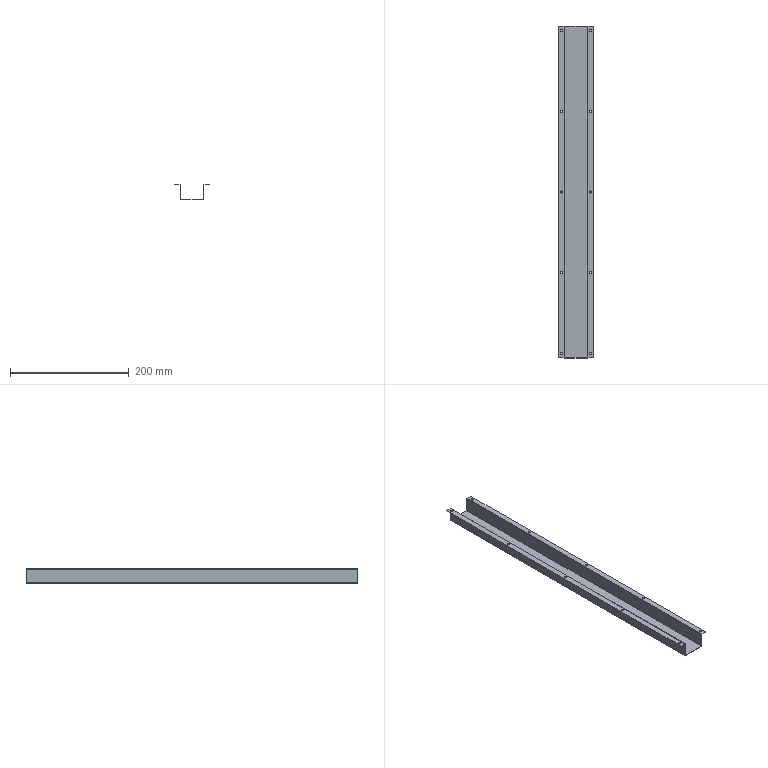Part | SolidWorks | features BaseBody 1 | 1 solid | 42 faces | box 58.8 x 560 x 25 mm | volume 35807 mm3 | cylinder 28 | plane 14 | commonest cylinder face diameters 3.5 x20 0.4 x4 1.6 x4
STEP:
#1=CARTESIAN_POINT('',(322.65,272.,-1.2));
#2=VERTEX_POINT('',#1);
#3=CARTESIAN_POINT('',(326.15,272.,-1.2));
#4=VERTEX_POINT('',#3);
#5=CARTESIAN_POINT('',(324.4,272.,-1.2));
#6=DIRECTION('',(0.,0.,1.));
#7=DIRECTION('',(1.,0.,0.));
#8=AXIS2_PLACEMENT_3D('',#5,#6,#7);
#9=CIRCLE('',#8,1.75);
#10=EDGE_CURVE('',#2,#4,#9,.T.);
#11=ORIENTED_EDGE('',*,*,#10,.F.);
#12=CARTESIAN_POINT('',(322.65,272.,-0.6));
#13=VERTEX_POINT('',#12);
#14=CARTESIAN_POINT('',(322.65,272.,-1.2));
#15=DIRECTION('',(0.,0.,1.));
#16=VECTOR('',#15,1000.);
#17=LINE('',#14,#16);
#18=EDGE_CURVE('',#2,#13,#17,.T.);
#19=ORIENTED_EDGE('',*,*,#18,.T.);
#20=CARTESIAN_POINT('',(326.15,272.,-0.6));
#21=VERTEX_POINT('',#20);
#22=CARTESIAN_POINT('',(324.4,272.,-0.6));
#23=DIRECTION('',(0.,0.,-1.));
#24=DIRECTION('',(1.,0.,0.));
#25=AXIS2_PLACEMENT_3D('',#22,#23,#24);
#26=CIRCLE('',#25,1.75);
#27=EDGE_CURVE('',#21,#13,#26,.T.);
#28=ORIENTED_EDGE('',*,*,#27,.F.);
#29=CARTESIAN_POINT('',(326.15,272.,-1.2));
#30=DIRECTION('',(0.,0.,1.));
#31=VECTOR('',#30,1000.);
#32=LINE('',#29,#31);
#33=EDGE_CURVE('',#4,#21,#32,.T.);
#34=ORIENTED_EDGE('',*,*,#33,.F.);
#35=EDGE_LOOP('',(#11,#19,#28,#34));
#36=FACE_OUTER_BOUND('',#35,.T.);
#37=CARTESIAN_POINT('',(324.4,272.,-1.2));
#38=DIRECTION('',(0.,0.,1.));
#39=DIRECTION('',(1.,0.,0.));
#40=AXIS2_PLACEMENT_3D('',#37,#38,#39);
#41=CYLINDRICAL_SURFACE('',#40,1.75);
#42=ADVANCED_FACE('',(#36),#41,.F.);
#43=CARTESIAN_POINT('',(322.65,0.,-1.2));
#44=VERTEX_POINT('',#43);
#45=CARTESIAN_POINT('',(326.15,0.,-1.2));
#46=VERTEX_POINT('',#45);
#47=CARTESIAN_POINT('',(324.4,0.,-1.2));
#48=DIRECTION('',(0.,0.,1.));
#49=DIRECTION('',(1.,0.,0.));
#50=AXIS2_PLACEMENT_3D('',#47,#48,#49);
#51=CIRCLE('',#50,1.75);
#52=EDGE_CURVE('',#44,#46,#51,.T.);
#53=ORIENTED_EDGE('',*,*,#52,.F.);
#54=CARTESIAN_POINT('',(322.65,0.,-0.6));
#55=VERTEX_POINT('',#54);
#56=CARTESIAN_POINT('',(322.65,0.,-1.2));
#57=DIRECTION('',(0.,0.,1.));
#58=VECTOR('',#57,1000.);
#59=LINE('',#56,#58);
#60=EDGE_CURVE('',#44,#55,#59,.T.);
#61=ORIENTED_EDGE('',*,*,#60,.T.);
#62=CARTESIAN_POINT('',(326.15,0.,-0.6));
#63=VERTEX_POINT('',#62);
#64=CARTESIAN_POINT('',(324.4,0.,-0.6));
#65=DIRECTION('',(0.,0.,-1.));
#66=DIRECTION('',(1.,0.,0.));
#67=AXIS2_PLACEMENT_3D('',#64,#65,#66);
#68=CIRCLE('',#67,1.75);
#69=EDGE_CURVE('',#63,#55,#68,.T.);
#70=ORIENTED_EDGE('',*,*,#69,.F.);
#71=CARTESIAN_POINT('',(326.15,0.,-1.2));
#72=DIRECTION('',(0.,0.,1.));
#73=VECTOR('',#72,1000.);
#74=LINE('',#71,#73);
#75=EDGE_CURVE('',#46,#63,#74,.T.);
#76=ORIENTED_EDGE('',*,*,#75,.F.);
#77=EDGE_LOOP('',(#53,#61,#70,#76));
#78=FACE_OUTER_BOUND('',#77,.T.);
#79=CARTESIAN_POINT('',(324.4,0.,-1.2));
#80=DIRECTION('',(0.,0.,1.));
#81=DIRECTION('',(1.,0.,0.));
#82=AXIS2_PLACEMENT_3D('',#79,#80,#81);
#83=CYLINDRICAL_SURFACE('',#82,1.75);
#84=ADVANCED_FACE('',(#78),#83,.F.);
#85=CARTESIAN_POINT('',(322.65,136.,-1.2));
#86=VERTEX_POINT('',#85);
#87=CARTESIAN_POINT('',(326.15,136.,-1.2));
#88=VERTEX_POINT('',#87);
#89=CARTESIAN_POINT('',(324.4,136.,-1.2));
#90=DIRECTION('',(0.,0.,1.));
#91=DIRECTION('',(1.,0.,0.));
#92=AXIS2_PLACEMENT_3D('',#89,#90,#91);
#93=CIRCLE('',#92,1.75);
#94=EDGE_CURVE('',#86,#88,#93,.T.);
#95=ORIENTED_EDGE('',*,*,#94,.F.);
#96=CARTESIAN_POINT('',(322.65,136.,-0.6));
#97=VERTEX_POINT('',#96);
#98=CARTESIAN_POINT('',(322.65,136.,-1.2));
#99=DIRECTION('',(0.,0.,1.));
#100=VECTOR('',#99,1000.);
#101=LINE('',#98,#100);
#102=EDGE_CURVE('',#86,#97,#101,.T.);
#103=ORIENTED_EDGE('',*,*,#102,.T.);
#104=CARTESIAN_POINT('',(326.15,136.,-0.6));
#105=VERTEX_POINT('',#104);
#106=CARTESIAN_POINT('',(324.4,136.,-0.6));
#107=DIRECTION('',(0.,0.,-1.));
#108=DIRECTION('',(1.,0.,0.));
#109=AXIS2_PLACEMENT_3D('',#106,#107,#108);
#110=CIRCLE('',#109,1.75);
#111=EDGE_CURVE('',#105,#97,#110,.T.);
#112=ORIENTED_EDGE('',*,*,#111,.F.);
#113=CARTESIAN_POINT('',(326.15,136.,-1.2));
#114=DIRECTION('',(0.,0.,1.));
#115=VECTOR('',#114,1000.);
#116=LINE('',#113,#115);
#117=EDGE_CURVE('',#88,#105,#116,.T.);
#118=ORIENTED_EDGE('',*,*,#117,.F.);
#119=EDGE_LOOP('',(#95,#103,#112,#118));
#120=FACE_OUTER_BOUND('',#119,.T.);
#121=CARTESIAN_POINT('',(324.4,136.,-1.2));
#122=DIRECTION('',(0.,0.,1.));
#123=DIRECTION('',(1.,0.,0.));
#124=AXIS2_PLACEMENT_3D('',#121,#122,#123);
#125=CYLINDRICAL_SURFACE('',#124,1.75);
#126=ADVANCED_FACE('',(#120),#125,.F.);
#127=CARTESIAN_POINT('',(322.65,-272.,-1.2));
#128=VERTEX_POINT('',#127);
#129=CARTESIAN_POINT('',(326.15,-272.,-1.2));
#130=VERTEX_POINT('',#129);
#131=CARTESIAN_POINT('',(324.4,-272.,-1.2));
#132=DIRECTION('',(0.,0.,1.));
#133=DIRECTION('',(1.,0.,0.));
#134=AXIS2_PLACEMENT_3D('',#131,#132,#133);
#135=CIRCLE('',#134,1.75);
#136=EDGE_CURVE('',#128,#130,#135,.T.);
#137=ORIENTED_EDGE('',*,*,#136,.F.);
#138=CARTESIAN_POINT('',(322.65,-272.,-0.6));
#139=VERTEX_POINT('',#138);
#140=CARTESIAN_POINT('',(322.65,-272.,-1.2));
#141=DIRECTION('',(0.,0.,1.));
#142=VECTOR('',#141,1000.);
#143=LINE('',#140,#142);
#144=EDGE_CURVE('',#128,#139,#143,.T.);
#145=ORIENTED_EDGE('',*,*,#144,.T.);
#146=CARTESIAN_POINT('',(326.15,-272.,-0.6));
#147=VERTEX_POINT('',#146);
#148=CARTESIAN_POINT('',(324.4,-272.,-0.6));
#149=DIRECTION('',(0.,0.,-1.));
#150=DIRECTION('',(1.,0.,0.));
#151=AXIS2_PLACEMENT_3D('',#148,#149,#150);
#152=CIRCLE('',#151,1.75);
#153=EDGE_CURVE('',#147,#139,#152,.T.);
#154=ORIENTED_EDGE('',*,*,#153,.F.);
#155=CARTESIAN_POINT('',(326.15,-272.,-1.2));
#156=DIRECTION('',(0.,0.,1.));
#157=VECTOR('',#156,1000.);
#158=LINE('',#155,#157);
#159=EDGE_CURVE('',#130,#147,#158,.T.);
#160=ORIENTED_EDGE('',*,*,#159,.F.);
#161=EDGE_LOOP('',(#137,#145,#154,#160));
#162=FACE_OUTER_BOUND('',#161,.T.);
#163=CARTESIAN_POINT('',(324.4,-272.,-1.2));
#164=DIRECTION('',(0.,0.,1.));
#165=DIRECTION('',(1.,0.,0.));
#166=AXIS2_PLACEMENT_3D('',#163,#164,#165);
#167=CYLINDRICAL_SURFACE('',#166,1.75);
#168=ADVANCED_FACE('',(#162),#167,.F.);
#169=CARTESIAN_POINT('',(322.65,-136.,-1.2));
#170=VERTEX_POINT('',#169);
#171=CARTESIAN_POINT('',(326.15,-136.,-1.2));
#172=VERTEX_POINT('',#171);
#173=CARTESIAN_POINT('',(324.4,-136.,-1.2));
#174=DIRECTION('',(0.,0.,1.));
#175=DIRECTION('',(1.,0.,0.));
#176=AXIS2_PLACEMENT_3D('',#173,#174,#175);
#177=CIRCLE('',#176,1.75);
#178=EDGE_CURVE('',#170,#172,#177,.T.);
#179=ORIENTED_EDGE('',*,*,#178,.F.);
#180=CARTESIAN_POINT('',(322.65,-136.,-0.6));
#181=VERTEX_POINT('',#180);
#182=CARTESIAN_POINT('',(322.65,-136.,-1.2));
#183=DIRECTION('',(0.,0.,1.));
#184=VECTOR('',#183,1000.);
#185=LINE('',#182,#184);
#186=EDGE_CURVE('',#170,#181,#185,.T.);
#187=ORIENTED_EDGE('',*,*,#186,.T.);
#188=CARTESIAN_POINT('',(326.15,-136.,-0.6));
#189=VERTEX_POINT('',#188);
#190=CARTESIAN_POINT('',(324.4,-136.,-0.6));
#191=DIRECTION('',(0.,0.,-1.));
#192=DIRECTION('',(1.,0.,0.));
#193=AXIS2_PLACEMENT_3D('',#190,#191,#192);
#194=CIRCLE('',#193,1.75);
#195=EDGE_CURVE('',#189,#181,#194,.T.);
#196=ORIENTED_EDGE('',*,*,#195,.F.);
#197=CARTESIAN_POINT('',(326.15,-136.,-1.2));
#198=DIRECTION('',(0.,0.,1.));
#199=VECTOR('',#198,1000.);
#200=LINE('',#197,#199);
#201=EDGE_CURVE('',#172,#189,#200,.T.);
#202=ORIENTED_EDGE('',*,*,#201,.F.);
#203=EDGE_LOOP('',(#179,#187,#196,#202));
#204=FACE_OUTER_BOUND('',#203,.T.);
#205=CARTESIAN_POINT('',(324.4,-136.,-1.2));
#206=DIRECTION('',(0.,0.,1.));
#207=DIRECTION('',(1.,0.,0.));
#208=AXIS2_PLACEMENT_3D('',#205,#206,#207);
#209=CYLINDRICAL_SURFACE('',#208,1.75);
#210=ADVANCED_FACE('',(#204),#209,.F.);
#211=CARTESIAN_POINT('',(273.85,-272.,-1.2));
#212=VERTEX_POINT('',#211);
#213=CARTESIAN_POINT('',(277.35,-272.,-1.2));
#214=VERTEX_POINT('',#213);
#215=CARTESIAN_POINT('',(275.6,-272.,-1.2));
#216=DIRECTION('',(0.,0.,1.));
#217=DIRECTION('',(1.,0.,0.));
#218=AXIS2_PLACEMENT_3D('',#215,#216,#217);
#219=CIRCLE('',#218,1.75);
#220=EDGE_CURVE('',#212,#214,#219,.T.);
#221=ORIENTED_EDGE('',*,*,#220,.F.);
#222=CARTESIAN_POINT('',(273.85,-272.,-0.6));
#223=VERTEX_POINT('',#222);
#224=CARTESIAN_POINT('',(273.85,-272.,-1.2));
#225=DIRECTION('',(0.,0.,1.));
#226=VECTOR('',#225,1000.);
#227=LINE('',#224,#226);
#228=EDGE_CURVE('',#212,#223,#227,.T.);
#229=ORIENTED_EDGE('',*,*,#228,.T.);
#230=CARTESIAN_POINT('',(277.35,-272.,-0.6));
#231=VERTEX_POINT('',#230);
#232=CARTESIAN_POINT('',(275.6,-272.,-0.6));
#233=DIRECTION('',(0.,0.,-1.));
#234=DIRECTION('',(1.,0.,0.));
#235=AXIS2_PLACEMENT_3D('',#232,#233,#234);
#236=CIRCLE('',#235,1.75);
#237=EDGE_CURVE('',#231,#223,#236,.T.);
#238=ORIENTED_EDGE('',*,*,#237,.F.);
#239=CARTESIAN_POINT('',(277.35,-272.,-1.2));
#240=DIRECTION('',(0.,0.,1.));
#241=VECTOR('',#240,1000.);
#242=LINE('',#239,#241);
#243=EDGE_CURVE('',#214,#231,#242,.T.);
#244=ORIENTED_EDGE('',*,*,#243,.F.);
#245=EDGE_LOOP('',(#221,#229,#238,#244));
#246=FACE_OUTER_BOUND('',#245,.T.);
#247=CARTESIAN_POINT('',(275.6,-272.,-1.2));
#248=DIRECTION('',(0.,0.,1.));
#249=DIRECTION('',(1.,0.,0.));
#250=AXIS2_PLACEMENT_3D('',#247,#248,#249);
#251=CYLINDRICAL_SURFACE('',#250,1.75);
#252=ADVANCED_FACE('',(#246),#251,.F.);
#253=CARTESIAN_POINT('',(273.85,136.,-1.2));
#254=VERTEX_POINT('',#253);
#255=CARTESIAN_POINT('',(277.35,136.,-1.2));
#256=VERTEX_POINT('',#255);
#257=CARTESIAN_POINT('',(275.6,136.,-1.2));
#258=DIRECTION('',(0.,0.,1.));
#259=DIRECTION('',(1.,0.,0.));
#260=AXIS2_PLACEMENT_3D('',#257,#258,#259);
#261=CIRCLE('',#260,1.75);
#262=EDGE_CURVE('',#254,#256,#261,.T.);
#263=ORIENTED_EDGE('',*,*,#262,.F.);
#264=CARTESIAN_POINT('',(273.85,136.,-0.6));
#265=VERTEX_POINT('',#264);
#266=CARTESIAN_POINT('',(273.85,136.,-1.2));
#267=DIRECTION('',(0.,0.,1.));
#268=VECTOR('',#267,1000.);
#269=LINE('',#266,#268);
#270=EDGE_CURVE('',#254,#265,#269,.T.);
#271=ORIENTED_EDGE('',*,*,#270,.T.);
#272=CARTESIAN_POINT('',(277.35,136.,-0.6));
#273=VERTEX_POINT('',#272);
#274=CARTESIAN_POINT('',(275.6,136.,-0.6));
#275=DIRECTION('',(0.,0.,-1.));
#276=DIRECTION('',(1.,0.,0.));
#277=AXIS2_PLACEMENT_3D('',#274,#275,#276);
#278=CIRCLE('',#277,1.75);
#279=EDGE_CURVE('',#273,#265,#278,.T.);
#280=ORIENTED_EDGE('',*,*,#279,.F.);
#281=CARTESIAN_POINT('',(277.35,136.,-1.2));
#282=DIRECTION('',(0.,0.,1.));
#283=VECTOR('',#282,1000.);
#284=LINE('',#281,#283);
#285=EDGE_CURVE('',#256,#273,#284,.T.);
#286=ORIENTED_EDGE('',*,*,#285,.F.);
#287=EDGE_LOOP('',(#263,#271,#280,#286));
#288=FACE_OUTER_BOUND('',#287,.T.);
#289=CARTESIAN_POINT('',(275.6,136.,-1.2));
#290=DIRECTION('',(0.,0.,1.));
#291=DIRECTION('',(1.,0.,0.));
#292=AXIS2_PLACEMENT_3D('',#289,#290,#291);
#293=CYLINDRICAL_SURFACE('',#292,1.75);
#294=ADVANCED_FACE('',(#288),#293,.F.);
#295=CARTESIAN_POINT('',(273.85,272.,-1.2));
#296=VERTEX_POINT('',#295);
#297=CARTESIAN_POINT('',(277.35,272.,-1.2));
#298=VERTEX_POINT('',#297);
#299=CARTESIAN_POINT('',(275.6,272.,-1.2));
#300=DIRECTION('',(0.,0.,1.));
#301=DIRECTION('',(1.,0.,0.));
#302=AXIS2_PLACEMENT_3D('',#299,#300,#301);
#303=CIRCLE('',#302,1.75);
#304=EDGE_CURVE('',#296,#298,#303,.T.);
#305=ORIENTED_EDGE('',*,*,#304,.F.);
#306=CARTESIAN_POINT('',(273.85,272.,-0.6));
#307=VERTEX_POINT('',#306);
#308=CARTESIAN_POINT('',(273.85,272.,-1.2));
#309=DIRECTION('',(0.,0.,1.));
#310=VECTOR('',#309,1000.);
#311=LINE('',#308,#310);
#312=EDGE_CURVE('',#296,#307,#311,.T.);
#313=ORIENTED_EDGE('',*,*,#312,.T.);
#314=CARTESIAN_POINT('',(277.35,272.,-0.6));
#315=VERTEX_POINT('',#314);
#316=CARTESIAN_POINT('',(275.6,272.,-0.6));
#317=DIRECTION('',(0.,0.,-1.));
#318=DIRECTION('',(1.,0.,0.));
#319=AXIS2_PLACEMENT_3D('',#316,#317,#318);
#320=CIRCLE('',#319,1.75);
#321=EDGE_CURVE('',#315,#307,#320,.T.);
#322=ORIENTED_EDGE('',*,*,#321,.F.);
#323=CARTESIAN_POINT('',(277.35,272.,-1.2));
#324=DIRECTION('',(0.,0.,1.));
#325=VECTOR('',#324,1000.);
#326=LINE('',#323,#325);
#327=EDGE_CURVE('',#298,#315,#326,.T.);
#328=ORIENTED_EDGE('',*,*,#327,.F.);
#329=EDGE_LOOP('',(#305,#313,#322,#328));
#330=FACE_OUTER_BOUND('',#329,.T.);
#331=CARTESIAN_POINT('',(275.6,272.,-1.2));
#332=DIRECTION('',(0.,0.,1.));
#333=DIRECTION('',(1.,0.,0.));
#334=AXIS2_PLACEMENT_3D('',#331,#332,#333);
#335=CYLINDRICAL_SURFACE('',#334,1.75);
#336=ADVANCED_FACE('',(#330),#335,.F.);
#337=CARTESIAN_POINT('',(273.85,-136.,-1.2));
#338=VERTEX_POINT('',#337);
#339=CARTESIAN_POINT('',(277.35,-136.,-1.2));
#340=VERTEX_POINT('',#339);
#341=CARTESIAN_POINT('',(275.6,-136.,-1.2));
#342=DIRECTION('',(0.,0.,1.));
#343=DIRECTION('',(1.,0.,0.));
#344=AXIS2_PLACEMENT_3D('',#341,#342,#343);
#345=CIRCLE('',#344,1.75);
#346=EDGE_CURVE('',#338,#340,#345,.T.);
#347=ORIENTED_EDGE('',*,*,#346,.F.);
#348=CARTESIAN_POINT('',(273.85,-136.,-0.6));
#349=VERTEX_POINT('',#348);
#350=CARTESIAN_POINT('',(273.85,-136.,-1.2));
#351=DIRECTION('',(0.,0.,1.));
#352=VECTOR('',#351,1000.);
#353=LINE('',#350,#352);
#354=EDGE_CURVE('',#338,#349,#353,.T.);
#355=ORIENTED_EDGE('',*,*,#354,.T.);
#356=CARTESIAN_POINT('',(277.35,-136.,-0.6));
#357=VERTEX_POINT('',#356);
#358=CARTESIAN_POINT('',(275.6,-136.,-0.6));
#359=DIRECTION('',(0.,0.,-1.));
#360=DIRECTION('',(1.,0.,0.));
#361=AXIS2_PLACEMENT_3D('',#358,#359,#360);
#362=CIRCLE('',#361,1.75);
#363=EDGE_CURVE('',#357,#349,#362,.T.);
#364=ORIENTED_EDGE('',*,*,#363,.F.);
#365=CARTESIAN_POINT('',(277.35,-136.,-1.2));
#366=DIRECTION('',(0.,0.,1.));
#367=VECTOR('',#366,1000.);
#368=LINE('',#365,#367);
#369=EDGE_CURVE('',#340,#357,#368,.T.);
#370=ORIENTED_EDGE('',*,*,#369,.F.);
#371=EDGE_LOOP('',(#347,#355,#364,#370));
#372=FACE_OUTER_BOUND('',#371,.T.);
#373=CARTESIAN_POINT('',(275.6,-136.,-1.2));
#374=DIRECTION('',(0.,0.,1.));
#375=DIRECTION('',(1.,0.,0.));
#376=AXIS2_PLACEMENT_3D('',#373,#374,#375);
#377=CYLINDRICAL_SURFACE('',#376,1.75);
#378=ADVANCED_FACE('',(#372),#377,.F.);
#379=CARTESIAN_POINT('',(273.85,0.,-1.2));
#380=VERTEX_POINT('',#379);
#381=CARTESIAN_POINT('',(277.35,0.,-1.2));
#382=VERTEX_POINT('',#381);
#383=CARTESIAN_POINT('',(275.6,0.,-1.2));
#384=DIRECTION('',(0.,0.,1.));
#385=DIRECTION('',(1.,0.,0.));
#386=AXIS2_PLACEMENT_3D('',#383,#384,#385);
#387=CIRCLE('',#386,1.75);
#388=EDGE_CURVE('',#380,#382,#387,.T.);
#389=ORIENTED_EDGE('',*,*,#388,.F.);
#390=CARTESIAN_POINT('',(273.85,0.,-0.6));
#391=VERTEX_POINT('',#390);
#392=CARTESIAN_POINT('',(273.85,0.,-1.2));
#393=DIRECTION('',(0.,0.,1.));
#394=VECTOR('',#393,1000.);
#395=LINE('',#392,#394);
#396=EDGE_CURVE('',#380,#391,#395,.T.);
#397=ORIENTED_EDGE('',*,*,#396,.T.);
#398=CARTESIAN_POINT('',(277.35,0.,-0.6));
#399=VERTEX_POINT('',#398);
#400=CARTESIAN_POINT('',(275.6,0.,-0.6));
#401=DIRECTION('',(0.,0.,-1.));
#402=DIRECTION('',(1.,0.,0.));
#403=AXIS2_PLACEMENT_3D('',#400,#401,#402);
#404=CIRCLE('',#403,1.75);
#405=EDGE_CURVE('',#399,#391,#404,.T.);
#406=ORIENTED_EDGE('',*,*,#405,.F.);
#407=CARTESIAN_POINT('',(277.35,0.,-1.2));
#408=DIRECTION('',(0.,0.,1.));
#409=VECTOR('',#408,1000.);
#410=LINE('',#407,#409);
#411=EDGE_CURVE('',#382,#399,#410,.T.);
#412=ORIENTED_EDGE('',*,*,#411,.F.);
#413=EDGE_LOOP('',(#389,#397,#406,#412));
#414=FACE_OUTER_BOUND('',#413,.T.);
#415=CARTESIAN_POINT('',(275.6,0.,-1.2));
#416=DIRECTION('',(0.,0.,1.));
#417=DIRECTION('',(1.,0.,0.));
#418=AXIS2_PLACEMENT_3D('',#415,#416,#417);
#419=CYLINDRICAL_SURFACE('',#418,1.75);
#420=ADVANCED_FACE('',(#414),#419,.F.);
#421=CARTESIAN_POINT('',(280.8,280.,-25.6));
#422=VERTEX_POINT('',#421);
#423=CARTESIAN_POINT('',(319.2,280.,-25.6));
#424=VERTEX_POINT('',#423);
#425=CARTESIAN_POINT('',(280.6,280.,-25.6));
#426=DIRECTION('',(1.,0.,0.));
#427=VECTOR('',#426,1000.);
#428=LINE('',#425,#427);
#429=EDGE_CURVE('',#422,#424,#428,.T.);
#430=ORIENTED_EDGE('',*,*,#429,.T.);
#431=CARTESIAN_POINT('',(319.2,-280.,-25.6));
#432=VERTEX_POINT('',#431);
#433=CARTESIAN_POINT('',(319.2,280.,-25.6));
#434=DIRECTION('',(0.,-1.,0.));
#435=VECTOR('',#434,1000.);
#436=LINE('',#433,#435);
#437=EDGE_CURVE('',#424,#432,#436,.T.);
#438=ORIENTED_EDGE('',*,*,#437,.T.);
#439=CARTESIAN_POINT('',(280.8,-280.,-25.6));
#440=VERTEX_POINT('',#439);
#441=CARTESIAN_POINT('',(280.6,-280.,-25.6));
#442=DIRECTION('',(-1.,0.,0.));
#443=VECTOR('',#442,1000.);
#444=LINE('',#441,#443);
#445=EDGE_CURVE('',#432,#440,#444,.T.);
#446=ORIENTED_EDGE('',*,*,#445,.T.);
#447=CARTESIAN_POINT('',(280.8,280.,-25.6));
#448=DIRECTION('',(0.,1.,0.));
#449=VECTOR('',#448,1000.);
#450=LINE('',#447,#449);
#451=EDGE_CURVE('',#440,#422,#450,.T.);
#452=ORIENTED_EDGE('',*,*,#451,.T.);
#453=EDGE_LOOP('',(#430,#438,#446,#452));
#454=FACE_OUTER_BOUND('',#453,.T.);
#455=CARTESIAN_POINT('',(280.6,280.,-25.6));
#456=DIRECTION('',(0.,0.,-1.));
#457=DIRECTION('',(-1.,0.,0.));
#458=AXIS2_PLACEMENT_3D('',#455,#456,#457);
#459=PLANE('',#458);
#460=ADVANCED_FACE('',(#454),#459,.T.);
#461=CARTESIAN_POINT('',(320.,280.,-24.8));
#462=VERTEX_POINT('',#461);
#463=CARTESIAN_POINT('',(319.2,280.,-24.8));
#464=DIRECTION('',(0.,-1.,0.));
#465=DIRECTION('',(0.,0.,-1.));
#466=AXIS2_PLACEMENT_3D('',#463,#464,#465);
#467=CIRCLE('',#466,0.8);
#468=EDGE_CURVE('',#424,#462,#467,.T.);
#469=ORIENTED_EDGE('',*,*,#468,.T.);
#470=CARTESIAN_POINT('',(320.,-280.,-24.8));
#471=VERTEX_POINT('',#470);
#472=CARTESIAN_POINT('',(320.,280.,-24.8));
#473=DIRECTION('',(0.,-1.,0.));
#474=VECTOR('',#473,1000.);
#475=LINE('',#472,#474);
#476=EDGE_CURVE('',#462,#471,#475,.T.);
#477=ORIENTED_EDGE('',*,*,#476,.T.);
#478=CARTESIAN_POINT('',(319.2,-280.,-24.8));
#479=DIRECTION('',(0.,1.,0.));
#480=DIRECTION('',(0.,0.,-1.));
#481=AXIS2_PLACEMENT_3D('',#478,#479,#480);
#482=CIRCLE('',#481,0.8);
#483=EDGE_CURVE('',#471,#432,#482,.T.);
#484=ORIENTED_EDGE('',*,*,#483,.T.);
#485=ORIENTED_EDGE('',*,*,#437,.F.);
#486=EDGE_LOOP('',(#469,#477,#484,#485));
#487=FACE_OUTER_BOUND('',#486,.T.);
#488=CARTESIAN_POINT('',(319.2,280.,-24.8));
#489=DIRECTION('',(0.,-1.,0.));
#490=DIRECTION('',(0.,0.,-1.));
#491=AXIS2_PLACEMENT_3D('',#488,#489,#490);
#492=CYLINDRICAL_SURFACE('',#491,0.8);
#493=ADVANCED_FACE('',(#487),#492,.T.);
#494=ORIENTED_EDGE('',*,*,#429,.F.);
#495=CARTESIAN_POINT('',(280.,280.,-24.8));
#496=VERTEX_POINT('',#495);
#497=CARTESIAN_POINT('',(280.8,280.,-24.8));
#498=DIRECTION('',(0.,-1.,0.));
#499=DIRECTION('',(0.,0.,-1.));
#500=AXIS2_PLACEMENT_3D('',#497,#498,#499);
#501=CIRCLE('',#500,0.8);
#502=EDGE_CURVE('',#496,#422,#501,.T.);
#503=ORIENTED_EDGE('',*,*,#502,.F.);
#504=CARTESIAN_POINT('',(280.,280.,-1.4));
#505=VERTEX_POINT('',#504);
#506=CARTESIAN_POINT('',(280.,280.,-0.6));
#507=DIRECTION('',(0.,0.,-1.));
#508=VECTOR('',#507,1000.);
#509=LINE('',#506,#508);
#510=EDGE_CURVE('',#505,#496,#509,.T.);
#511=ORIENTED_EDGE('',*,*,#510,.F.);
#512=CARTESIAN_POINT('',(279.8,280.,-1.2));
#513=VERTEX_POINT('',#512);
#514=CARTESIAN_POINT('',(279.8,280.,-1.4));
#515=DIRECTION('',(0.,-1.,0.));
#516=DIRECTION('',(0.,0.,-1.));
#517=AXIS2_PLACEMENT_3D('',#514,#515,#516);
#518=CIRCLE('',#517,0.2);
#519=EDGE_CURVE('',#505,#513,#518,.T.);
#520=ORIENTED_EDGE('',*,*,#519,.T.);
#521=CARTESIAN_POINT('',(270.6,280.,-1.2));
#522=VERTEX_POINT('',#521);
#523=CARTESIAN_POINT('',(270.6,280.,-1.2));
#524=DIRECTION('',(1.,0.,0.));
#525=VECTOR('',#524,1000.);
#526=LINE('',#523,#525);
#527=EDGE_CURVE('',#522,#513,#526,.T.);
#528=ORIENTED_EDGE('',*,*,#527,.F.);
#529=CARTESIAN_POINT('',(270.6,280.,-0.6));
#530=VERTEX_POINT('',#529);
#531=CARTESIAN_POINT('',(270.6,280.,-1.4));
#532=DIRECTION('',(0.,0.,1.));
#533=VECTOR('',#532,1000.);
#534=LINE('',#531,#533);
#535=EDGE_CURVE('',#522,#530,#534,.T.);
#536=ORIENTED_EDGE('',*,*,#535,.T.);
#537=CARTESIAN_POINT('',(279.8,280.,-0.6));
#538=VERTEX_POINT('',#537);
#539=CARTESIAN_POINT('',(280.,280.,-0.6));
#540=DIRECTION('',(1.,0.,0.));
#541=VECTOR('',#540,1000.);
#542=LINE('',#539,#541);
#543=EDGE_CURVE('',#530,#538,#542,.T.);
#544=ORIENTED_EDGE('',*,*,#543,.T.);
#545=CARTESIAN_POINT('',(280.6,280.,-1.4));
#546=VERTEX_POINT('',#545);
#547=CARTESIAN_POINT('',(279.8,280.,-1.4));
#548=DIRECTION('',(0.,1.,0.));
#549=DIRECTION('',(0.,0.,-1.));
#550=AXIS2_PLACEMENT_3D('',#547,#548,#549);
#551=CIRCLE('',#550,0.8);
#552=EDGE_CURVE('',#538,#546,#551,.T.);
#553=ORIENTED_EDGE('',*,*,#552,.T.);
#554=CARTESIAN_POINT('',(280.6,280.,-24.8));
#555=VERTEX_POINT('',#554);
#556=CARTESIAN_POINT('',(280.6,280.,-25.6));
#557=DIRECTION('',(0.,0.,-1.));
#558=VECTOR('',#557,1000.);
#559=LINE('',#556,#558);
#560=EDGE_CURVE('',#546,#555,#559,.T.);
#561=ORIENTED_EDGE('',*,*,#560,.T.);
#562=CARTESIAN_POINT('',(280.8,280.,-25.));
#563=VERTEX_POINT('',#562);
#564=CARTESIAN_POINT('',(280.8,280.,-24.8));
#565=DIRECTION('',(0.,-1.,0.));
#566=DIRECTION('',(0.,0.,-1.));
#567=AXIS2_PLACEMENT_3D('',#564,#565,#566);
#568=CIRCLE('',#567,0.2);
#569=EDGE_CURVE('',#555,#563,#568,.T.);
#570=ORIENTED_EDGE('',*,*,#569,.T.);
#571=CARTESIAN_POINT('',(319.2,280.,-25.));
#572=VERTEX_POINT('',#571);
#573=CARTESIAN_POINT('',(320.,280.,-25.));
#574=DIRECTION('',(1.,0.,0.));
#575=VECTOR('',#574,1000.);
#576=LINE('',#573,#575);
#577=EDGE_CURVE('',#563,#572,#576,.T.);
#578=ORIENTED_EDGE('',*,*,#577,.T.);
#579=CARTESIAN_POINT('',(319.4,280.,-24.8));
#580=VERTEX_POINT('',#579);
#581=CARTESIAN_POINT('',(319.2,280.,-24.8));
#582=DIRECTION('',(0.,-1.,0.));
#583=DIRECTION('',(0.,0.,-1.));
#584=AXIS2_PLACEMENT_3D('',#581,#582,#583);
#585=CIRCLE('',#584,0.2);
#586=EDGE_CURVE('',#572,#580,#585,.T.);
#587=ORIENTED_EDGE('',*,*,#586,.T.);
#588=CARTESIAN_POINT('',(319.4,280.,-1.4));
#589=VERTEX_POINT('',#588);
#590=CARTESIAN_POINT('',(319.4,280.,-1.2));
#591=DIRECTION('',(0.,0.,1.));
#592=VECTOR('',#591,1000.);
#593=LINE('',#590,#592);
#594=EDGE_CURVE('',#580,#589,#593,.T.);
#595=ORIENTED_EDGE('',*,*,#594,.T.);
#596=CARTESIAN_POINT('',(320.2,280.,-0.6));
#597=VERTEX_POINT('',#596);
#598=CARTESIAN_POINT('',(320.2,280.,-1.4));
#599=DIRECTION('',(0.,-1.,0.));
#600=DIRECTION('',(0.,0.,-1.));
#601=AXIS2_PLACEMENT_3D('',#598,#599,#600);
#602=CIRCLE('',#601,0.8);
#603=EDGE_CURVE('',#597,#589,#602,.T.);
#604=ORIENTED_EDGE('',*,*,#603,.F.);
#605=CARTESIAN_POINT('',(329.4,280.,-0.6));
#606=VERTEX_POINT('',#605);
#607=CARTESIAN_POINT('',(320.2,280.,-0.6));
#608=DIRECTION('',(1.,0.,0.));
#609=VECTOR('',#608,1000.);
#610=LINE('',#607,#609);
#611=EDGE_CURVE('',#597,#606,#610,.T.);
#612=ORIENTED_EDGE('',*,*,#611,.T.);
#613=CARTESIAN_POINT('',(329.4,280.,-1.2));
#614=VERTEX_POINT('',#613);
#615=CARTESIAN_POINT('',(329.4,280.,-1.2));
#616=DIRECTION('',(0.,0.,1.));
#617=VECTOR('',#616,1000.);
#618=LINE('',#615,#617);
#619=EDGE_CURVE('',#614,#606,#618,.T.);
#620=ORIENTED_EDGE('',*,*,#619,.F.);
#621=CARTESIAN_POINT('',(320.2,280.,-1.2));
#622=VERTEX_POINT('',#621);
#623=CARTESIAN_POINT('',(319.4,280.,-1.2));
#624=DIRECTION('',(1.,0.,0.));
#625=VECTOR('',#624,1000.);
#626=LINE('',#623,#625);
#627=EDGE_CURVE('',#622,#614,#626,.T.);
#628=ORIENTED_EDGE('',*,*,#627,.F.);
#629=CARTESIAN_POINT('',(320.,280.,-1.4));
#630=VERTEX_POINT('',#629);
#631=CARTESIAN_POINT('',(320.2,280.,-1.4));
#632=DIRECTION('',(0.,-1.,0.));
#633=DIRECTION('',(0.,0.,-1.));
#634=AXIS2_PLACEMENT_3D('',#631,#632,#633);
#635=CIRCLE('',#634,0.2);
#636=EDGE_CURVE('',#622,#630,#635,.T.);
#637=ORIENTED_EDGE('',*,*,#636,.T.);
#638=CARTESIAN_POINT('',(320.,280.,-25.));
#639=DIRECTION('',(0.,0.,1.));
#640=VECTOR('',#639,1000.);
#641=LINE('',#638,#640);
#642=EDGE_CURVE('',#462,#630,#641,.T.);
#643=ORIENTED_EDGE('',*,*,#642,.F.);
#644=ORIENTED_EDGE('',*,*,#468,.F.);
#645=EDGE_LOOP('',(#494,#503,#511,#520,#528,#536,#544,#553,#561,#570,#578,#587,#595,#604,#612,#620,#628,#637,#643,#644));
#646=FACE_OUTER_BOUND('',#645,.T.);
#647=CARTESIAN_POINT('',(320.,280.,-24.8));
#648=DIRECTION('',(0.,1.,0.));
#649=DIRECTION('',(0.,0.,1.));
#650=AXIS2_PLACEMENT_3D('',#647,#648,#649);
#651=PLANE('',#650);
#652=ADVANCED_FACE('',(#646),#651,.T.);
#653=ORIENTED_EDGE('',*,*,#502,.T.);
#654=ORIENTED_EDGE('',*,*,#451,.F.);
#655=CARTESIAN_POINT('',(280.,-280.,-24.8));
#656=VERTEX_POINT('',#655);
#657=CARTESIAN_POINT('',(280.8,-280.,-24.8));
#658=DIRECTION('',(0.,1.,0.));
#659=DIRECTION('',(0.,0.,-1.));
#660=AXIS2_PLACEMENT_3D('',#657,#658,#659);
#661=CIRCLE('',#660,0.8);
#662=EDGE_CURVE('',#440,#656,#661,.T.);
#663=ORIENTED_EDGE('',*,*,#662,.T.);
#664=CARTESIAN_POINT('',(280.,280.,-24.8));
#665=DIRECTION('',(0.,1.,0.));
#666=VECTOR('',#665,1000.);
#667=LINE('',#664,#666);
#668=EDGE_CURVE('',#656,#496,#667,.T.);
#669=ORIENTED_EDGE('',*,*,#668,.T.);
#670=EDGE_LOOP('',(#653,#654,#663,#669));
#671=FACE_OUTER_BOUND('',#670,.T.);
#672=CARTESIAN_POINT('',(280.8,280.,-24.8));
#673=DIRECTION('',(0.,-1.,0.));
#674=DIRECTION('',(0.,0.,-1.));
#675=AXIS2_PLACEMENT_3D('',#672,#673,#674);
#676=CYLINDRICAL_SURFACE('',#675,0.8);
#677=ADVANCED_FACE('',(#671),#676,.T.);
#678=ORIENTED_EDGE('',*,*,#445,.F.);
#679=ORIENTED_EDGE('',*,*,#483,.F.);
#680=CARTESIAN_POINT('',(320.,-280.,-1.4));
#681=VERTEX_POINT('',#680);
#682=CARTESIAN_POINT('',(320.,-280.,-25.));
#683=DIRECTION('',(0.,0.,-1.));
#684=VECTOR('',#683,1000.);
#685=LINE('',#682,#684);
#686=EDGE_CURVE('',#681,#471,#685,.T.);
#687=ORIENTED_EDGE('',*,*,#686,.F.);
#688=CARTESIAN_POINT('',(320.2,-280.,-1.2));
#689=VERTEX_POINT('',#688);
#690=CARTESIAN_POINT('',(320.2,-280.,-1.4));
#691=DIRECTION('',(0.,1.,0.));
#692=DIRECTION('',(0.,0.,-1.));
#693=AXIS2_PLACEMENT_3D('',#690,#691,#692);
#694=CIRCLE('',#693,0.2);
#695=EDGE_CURVE('',#681,#689,#694,.T.);
#696=ORIENTED_EDGE('',*,*,#695,.T.);
#697=CARTESIAN_POINT('',(329.4,-280.,-1.2));
#698=VERTEX_POINT('',#697);
#699=CARTESIAN_POINT('',(319.4,-280.,-1.2));
#700=DIRECTION('',(-1.,0.,0.));
#701=VECTOR('',#700,1000.);
#702=LINE('',#699,#701);
#703=EDGE_CURVE('',#698,#689,#702,.T.);
#704=ORIENTED_EDGE('',*,*,#703,.F.);
#705=CARTESIAN_POINT('',(329.4,-280.,-0.6));
#706=VERTEX_POINT('',#705);
#707=CARTESIAN_POINT('',(329.4,-280.,-1.2));
#708=DIRECTION('',(0.,0.,-1.));
#709=VECTOR('',#708,1000.);
#710=LINE('',#707,#709);
#711=EDGE_CURVE('',#706,#698,#710,.T.);
#712=ORIENTED_EDGE('',*,*,#711,.F.);
#713=CARTESIAN_POINT('',(320.2,-280.,-0.6));
#714=VERTEX_POINT('',#713);
#715=CARTESIAN_POINT('',(320.,-280.,-0.6));
#716=DIRECTION('',(-1.,0.,0.));
#717=VECTOR('',#716,1000.);
#718=LINE('',#715,#717);
#719=EDGE_CURVE('',#706,#714,#718,.T.);
#720=ORIENTED_EDGE('',*,*,#719,.T.);
#721=CARTESIAN_POINT('',(319.4,-280.,-1.4));
#722=VERTEX_POINT('',#721);
#723=CARTESIAN_POINT('',(320.2,-280.,-1.4));
#724=DIRECTION('',(0.,1.,0.));
#725=DIRECTION('',(0.,0.,-1.));
#726=AXIS2_PLACEMENT_3D('',#723,#724,#725);
#727=CIRCLE('',#726,0.8);
#728=EDGE_CURVE('',#722,#714,#727,.T.);
#729=ORIENTED_EDGE('',*,*,#728,.F.);
#730=CARTESIAN_POINT('',(319.4,-280.,-24.8));
#731=VERTEX_POINT('',#730);
#732=CARTESIAN_POINT('',(319.4,-280.,-25.6));
#733=DIRECTION('',(0.,0.,-1.));
#734=VECTOR('',#733,1000.);
#735=LINE('',#732,#734);
#736=EDGE_CURVE('',#722,#731,#735,.T.);
#737=ORIENTED_EDGE('',*,*,#736,.T.);
#738=CARTESIAN_POINT('',(319.2,-280.,-25.));
#739=VERTEX_POINT('',#738);
#740=CARTESIAN_POINT('',(319.2,-280.,-24.8));
#741=DIRECTION('',(0.,1.,0.));
#742=DIRECTION('',(0.,0.,-1.));
#743=AXIS2_PLACEMENT_3D('',#740,#741,#742);
#744=CIRCLE('',#743,0.2);
#745=EDGE_CURVE('',#731,#739,#744,.T.);
#746=ORIENTED_EDGE('',*,*,#745,.T.);
#747=CARTESIAN_POINT('',(280.8,-280.,-25.));
#748=VERTEX_POINT('',#747);
#749=CARTESIAN_POINT('',(280.,-280.,-25.));
#750=DIRECTION('',(-1.,0.,0.));
#751=VECTOR('',#750,1000.);
#752=LINE('',#749,#751);
#753=EDGE_CURVE('',#739,#748,#752,.T.);
#754=ORIENTED_EDGE('',*,*,#753,.T.);
#755=CARTESIAN_POINT('',(280.6,-280.,-24.8));
#756=VERTEX_POINT('',#755);
#757=CARTESIAN_POINT('',(280.8,-280.,-24.8));
#758=DIRECTION('',(0.,1.,0.));
#759=DIRECTION('',(0.,0.,-1.));
#760=AXIS2_PLACEMENT_3D('',#757,#758,#759);
#761=CIRCLE('',#760,0.2);
#762=EDGE_CURVE('',#748,#756,#761,.T.);
#763=ORIENTED_EDGE('',*,*,#762,.T.);
#764=CARTESIAN_POINT('',(280.6,-280.,-1.4));
#765=VERTEX_POINT('',#764);
#766=CARTESIAN_POINT('',(280.6,-280.,-1.2));
#767=DIRECTION('',(0.,0.,1.));
#768=VECTOR('',#767,1000.);
#769=LINE('',#766,#768);
#770=EDGE_CURVE('',#756,#765,#769,.T.);
#771=ORIENTED_EDGE('',*,*,#770,.T.);
#772=CARTESIAN_POINT('',(279.8,-280.,-0.6));
#773=VERTEX_POINT('',#772);
#774=CARTESIAN_POINT('',(279.8,-280.,-1.4));
#775=DIRECTION('',(0.,-1.,0.));
#776=DIRECTION('',(0.,0.,-1.));
#777=AXIS2_PLACEMENT_3D('',#774,#775,#776);
#778=CIRCLE('',#777,0.8);
#779=EDGE_CURVE('',#765,#773,#778,.T.);
#780=ORIENTED_EDGE('',*,*,#779,.T.);
#781=CARTESIAN_POINT('',(270.6,-280.,-0.6));
#782=VERTEX_POINT('',#781);
#783=CARTESIAN_POINT('',(320.2,-280.,-0.6));
#784=DIRECTION('',(1.,0.,0.));
#785=VECTOR('',#784,1000.);
#786=LINE('',#783,#785);
#787=EDGE_CURVE('',#782,#773,#786,.T.);
#788=ORIENTED_EDGE('',*,*,#787,.F.);
#789=CARTESIAN_POINT('',(270.6,-280.,-1.2));
#790=VERTEX_POINT('',#789);
#791=CARTESIAN_POINT('',(270.6,-280.,-0.6));
#792=DIRECTION('',(0.,0.,1.));
#793=VECTOR('',#792,1000.);
#794=LINE('',#791,#793);
#795=EDGE_CURVE('',#790,#782,#794,.T.);
#796=ORIENTED_EDGE('',*,*,#795,.F.);
#797=CARTESIAN_POINT('',(279.8,-280.,-1.2));
#798=VERTEX_POINT('',#797);
#799=CARTESIAN_POINT('',(270.6,-280.,-1.2));
#800=DIRECTION('',(-1.,0.,0.));
#801=VECTOR('',#800,1000.);
#802=LINE('',#799,#801);
#803=EDGE_CURVE('',#798,#790,#802,.T.);
#804=ORIENTED_EDGE('',*,*,#803,.F.);
#805=CARTESIAN_POINT('',(280.,-280.,-1.4));
#806=VERTEX_POINT('',#805);
#807=CARTESIAN_POINT('',(279.8,-280.,-1.4));
#808=DIRECTION('',(0.,1.,0.));
#809=DIRECTION('',(0.,0.,-1.));
#810=AXIS2_PLACEMENT_3D('',#807,#808,#809);
#811=CIRCLE('',#810,0.2);
#812=EDGE_CURVE('',#798,#806,#811,.T.);
#813=ORIENTED_EDGE('',*,*,#812,.T.);
#814=CARTESIAN_POINT('',(280.,-280.,-0.6));
#815=DIRECTION('',(0.,0.,1.));
#816=VECTOR('',#815,1000.);
#817=LINE('',#814,#816);
#818=EDGE_CURVE('',#656,#806,#817,.T.);
#819=ORIENTED_EDGE('',*,*,#818,.F.);
#820=ORIENTED_EDGE('',*,*,#662,.F.);
#821=EDGE_LOOP('',(#678,#679,#687,#696,#704,#712,#720,#729,#737,#746,#754,#763,#771,#780,#788,#796,#804,#813,#819,#820));
#822=FACE_OUTER_BOUND('',#821,.T.);
#823=CARTESIAN_POINT('',(280.,-280.,-24.8));
#824=DIRECTION('',(0.,-1.,0.));
#825=DIRECTION('',(0.,0.,-1.));
#826=AXIS2_PLACEMENT_3D('',#823,#824,#825);
#827=PLANE('',#826);
#828=ADVANCED_FACE('',(#822),#827,.T.);
#829=ORIENTED_EDGE('',*,*,#642,.T.);
#830=CARTESIAN_POINT('',(320.,280.,-1.4));
#831=DIRECTION('',(0.,-1.,0.));
#832=VECTOR('',#831,1000.);
#833=LINE('',#830,#832);
#834=EDGE_CURVE('',#630,#681,#833,.T.);
#835=ORIENTED_EDGE('',*,*,#834,.T.);
#836=ORIENTED_EDGE('',*,*,#686,.T.);
#837=ORIENTED_EDGE('',*,*,#476,.F.);
#838=EDGE_LOOP('',(#829,#835,#836,#837));
#839=FACE_OUTER_BOUND('',#838,.T.);
#840=CARTESIAN_POINT('',(320.,280.,-25.));
#841=DIRECTION('',(1.,0.,0.));
#842=DIRECTION('',(0.,0.,-1.));
#843=AXIS2_PLACEMENT_3D('',#840,#841,#842);
#844=PLANE('',#843);
#845=ADVANCED_FACE('',(#839),#844,.T.);
#846=CARTESIAN_POINT('',(319.2,280.,-25.));
#847=DIRECTION('',(0.,-1.,0.));
#848=VECTOR('',#847,1000.);
#849=LINE('',#846,#848);
#850=EDGE_CURVE('',#572,#739,#849,.T.);
#851=ORIENTED_EDGE('',*,*,#850,.F.);
#852=ORIENTED_EDGE('',*,*,#577,.F.);
#853=CARTESIAN_POINT('',(280.8,280.,-25.));
#854=DIRECTION('',(0.,1.,0.));
#855=VECTOR('',#854,1000.);
#856=LINE('',#853,#855);
#857=EDGE_CURVE('',#748,#563,#856,.T.);
#858=ORIENTED_EDGE('',*,*,#857,.F.);
#859=ORIENTED_EDGE('',*,*,#753,.F.);
#860=EDGE_LOOP('',(#851,#852,#858,#859));
#861=FACE_OUTER_BOUND('',#860,.T.);
#862=CARTESIAN_POINT('',(280.6,280.,-25.));
#863=DIRECTION('',(0.,0.,-1.));
#864=DIRECTION('',(-1.,0.,0.));
#865=AXIS2_PLACEMENT_3D('',#862,#863,#864);
#866=PLANE('',#865);
#867=ADVANCED_FACE('',(#861),#866,.F.);
#868=ORIENTED_EDGE('',*,*,#510,.T.);
#869=ORIENTED_EDGE('',*,*,#668,.F.);
#870=ORIENTED_EDGE('',*,*,#818,.T.);
#871=CARTESIAN_POINT('',(280.,280.,-1.4));
#872=DIRECTION('',(0.,1.,0.));
#873=VECTOR('',#872,1000.);
#874=LINE('',#871,#873);
#875=EDGE_CURVE('',#806,#505,#874,.T.);
#876=ORIENTED_EDGE('',*,*,#875,.T.);
#877=EDGE_LOOP('',(#868,#869,#870,#876));
#878=FACE_OUTER_BOUND('',#877,.T.);
#879=CARTESIAN_POINT('',(280.,280.,-0.6));
#880=DIRECTION('',(-1.,0.,0.));
#881=DIRECTION('',(0.,0.,1.));
#882=AXIS2_PLACEMENT_3D('',#879,#880,#881);
#883=PLANE('',#882);
#884=ADVANCED_FACE('',(#878),#883,.T.);
#885=ORIENTED_EDGE('',*,*,#834,.F.);
#886=ORIENTED_EDGE('',*,*,#636,.F.);
#887=CARTESIAN_POINT('',(320.2,280.,-1.2));
#888=DIRECTION('',(0.,1.,0.));
#889=VECTOR('',#888,1000.);
#890=LINE('',#887,#889);
#891=EDGE_CURVE('',#689,#622,#890,.T.);
#892=ORIENTED_EDGE('',*,*,#891,.F.);
#893=ORIENTED_EDGE('',*,*,#695,.F.);
#894=EDGE_LOOP('',(#885,#886,#892,#893));
#895=FACE_OUTER_BOUND('',#894,.T.);
#896=CARTESIAN_POINT('',(320.2,280.,-1.4));
#897=DIRECTION('',(0.,-1.,0.));
#898=DIRECTION('',(0.,0.,-1.));
#899=AXIS2_PLACEMENT_3D('',#896,#897,#898);
#900=CYLINDRICAL_SURFACE('',#899,0.2);
#901=ADVANCED_FACE('',(#895),#900,.F.);
#902=CARTESIAN_POINT('',(319.4,280.,-24.8));
#903=DIRECTION('',(0.,-1.,0.));
#904=VECTOR('',#903,1000.);
#905=LINE('',#902,#904);
#906=EDGE_CURVE('',#580,#731,#905,.T.);
#907=ORIENTED_EDGE('',*,*,#906,.F.);
#908=ORIENTED_EDGE('',*,*,#586,.F.);
#909=ORIENTED_EDGE('',*,*,#850,.T.);
#910=ORIENTED_EDGE('',*,*,#745,.F.);
#911=EDGE_LOOP('',(#907,#908,#909,#910));
#912=FACE_OUTER_BOUND('',#911,.T.);
#913=CARTESIAN_POINT('',(319.2,280.,-24.8));
#914=DIRECTION('',(0.,-1.,0.));
#915=DIRECTION('',(0.,0.,-1.));
#916=AXIS2_PLACEMENT_3D('',#913,#914,#915);
#917=CYLINDRICAL_SURFACE('',#916,0.2);
#918=ADVANCED_FACE('',(#912),#917,.F.);
#919=ORIENTED_EDGE('',*,*,#857,.T.);
#920=ORIENTED_EDGE('',*,*,#569,.F.);
#921=CARTESIAN_POINT('',(280.6,280.,-24.8));
#922=DIRECTION('',(0.,1.,0.));
#923=VECTOR('',#922,1000.);
#924=LINE('',#921,#923);
#925=EDGE_CURVE('',#756,#555,#924,.T.);
#926=ORIENTED_EDGE('',*,*,#925,.F.);
#927=ORIENTED_EDGE('',*,*,#762,.F.);
#928=EDGE_LOOP('',(#919,#920,#926,#927));
#929=FACE_OUTER_BOUND('',#928,.T.);
#930=CARTESIAN_POINT('',(280.8,280.,-24.8));
#931=DIRECTION('',(0.,-1.,0.));
#932=DIRECTION('',(0.,0.,-1.));
#933=AXIS2_PLACEMENT_3D('',#930,#931,#932);
#934=CYLINDRICAL_SURFACE('',#933,0.2);
#935=ADVANCED_FACE('',(#929),#934,.F.);
#936=CARTESIAN_POINT('',(279.8,280.,-1.2));
#937=DIRECTION('',(0.,-1.,0.));
#938=VECTOR('',#937,1000.);
#939=LINE('',#936,#938);
#940=EDGE_CURVE('',#513,#798,#939,.T.);
#941=ORIENTED_EDGE('',*,*,#940,.F.);
#942=ORIENTED_EDGE('',*,*,#519,.F.);
#943=ORIENTED_EDGE('',*,*,#875,.F.);
#944=ORIENTED_EDGE('',*,*,#812,.F.);
#945=EDGE_LOOP('',(#941,#942,#943,#944));
#946=FACE_OUTER_BOUND('',#945,.T.);
#947=CARTESIAN_POINT('',(279.8,280.,-1.4));
#948=DIRECTION('',(0.,-1.,0.));
#949=DIRECTION('',(0.,0.,-1.));
#950=AXIS2_PLACEMENT_3D('',#947,#948,#949);
#951=CYLINDRICAL_SURFACE('',#950,0.2);
#952=ADVANCED_FACE('',(#946),#951,.F.);
#953=ORIENTED_EDGE('',*,*,#627,.T.);
#954=CARTESIAN_POINT('',(329.4,280.,-1.2));
#955=DIRECTION('',(0.,-1.,0.));
#956=VECTOR('',#955,1000.);
#957=LINE('',#954,#956);
#958=EDGE_CURVE('',#614,#698,#957,.T.);
#959=ORIENTED_EDGE('',*,*,#958,.T.);
#960=ORIENTED_EDGE('',*,*,#703,.T.);
#961=ORIENTED_EDGE('',*,*,#891,.T.);
#962=EDGE_LOOP('',(#953,#959,#960,#961));
#963=FACE_OUTER_BOUND('',#962,.T.);
#964=CARTESIAN_POINT('',(324.4,272.,-1.2));
#965=DIRECTION('',(0.,0.,1.));
#966=DIRECTION('',(1.,0.,0.));
#967=AXIS2_PLACEMENT_3D('',#964,#965,#966);
#968=CIRCLE('',#967,1.75);
#969=EDGE_CURVE('',#4,#2,#968,.T.);
#970=ORIENTED_EDGE('',*,*,#969,.T.);
#971=ORIENTED_EDGE('',*,*,#10,.T.);
#972=EDGE_LOOP('',(#970,#971));
#973=FACE_BOUND('',#972,.T.);
#974=CARTESIAN_POINT('',(324.4,0.,-1.2));
#975=DIRECTION('',(0.,0.,1.));
#976=DIRECTION('',(1.,0.,0.));
#977=AXIS2_PLACEMENT_3D('',#974,#975,#976);
#978=CIRCLE('',#977,1.75);
#979=EDGE_CURVE('',#46,#44,#978,.T.);
#980=ORIENTED_EDGE('',*,*,#979,.T.);
#981=ORIENTED_EDGE('',*,*,#52,.T.);
#982=EDGE_LOOP('',(#980,#981));
#983=FACE_BOUND('',#982,.T.);
#984=CARTESIAN_POINT('',(324.4,136.,-1.2));
#985=DIRECTION('',(0.,0.,1.));
#986=DIRECTION('',(1.,0.,0.));
#987=AXIS2_PLACEMENT_3D('',#984,#985,#986);
#988=CIRCLE('',#987,1.75);
#989=EDGE_CURVE('',#88,#86,#988,.T.);
#990=ORIENTED_EDGE('',*,*,#989,.T.);
#991=ORIENTED_EDGE('',*,*,#94,.T.);
#992=EDGE_LOOP('',(#990,#991));
#993=FACE_BOUND('',#992,.T.);
#994=CARTESIAN_POINT('',(324.4,-272.,-1.2));
#995=DIRECTION('',(0.,0.,1.));
#996=DIRECTION('',(1.,0.,0.));
#997=AXIS2_PLACEMENT_3D('',#994,#995,#996);
#998=CIRCLE('',#997,1.75);
#999=EDGE_CURVE('',#130,#128,#998,.T.);
#1000=ORIENTED_EDGE('',*,*,#999,.T.);
#1001=ORIENTED_EDGE('',*,*,#136,.T.);
#1002=EDGE_LOOP('',(#1000,#1001));
#1003=FACE_BOUND('',#1002,.T.);
#1004=CARTESIAN_POINT('',(324.4,-136.,-1.2));
#1005=DIRECTION('',(0.,0.,1.));
#1006=DIRECTION('',(1.,0.,0.));
#1007=AXIS2_PLACEMENT_3D('',#1004,#1005,#1006);
#1008=CIRCLE('',#1007,1.75);
#1009=EDGE_CURVE('',#172,#170,#1008,.T.);
#1010=ORIENTED_EDGE('',*,*,#1009,.T.);
#1011=ORIENTED_EDGE('',*,*,#178,.T.);
#1012=EDGE_LOOP('',(#1010,#1011));
#1013=FACE_BOUND('',#1012,.T.);
#1014=CARTESIAN_POINT('',(319.4,280.,-1.2));
#1015=DIRECTION('',(0.,0.,-1.));
#1016=DIRECTION('',(-1.,0.,0.));
#1017=AXIS2_PLACEMENT_3D('',#1014,#1015,#1016);
#1018=PLANE('',#1017);
#1019=ADVANCED_FACE('',(#963,#973,#983,#993,#1003,#1013),#1018,.T.);
#1020=CARTESIAN_POINT('',(319.4,280.,-1.4));
#1021=DIRECTION('',(0.,-1.,0.));
#1022=VECTOR('',#1021,1000.);
#1023=LINE('',#1020,#1022);
#1024=EDGE_CURVE('',#589,#722,#1023,.T.);
#1025=ORIENTED_EDGE('',*,*,#1024,.F.);
#1026=ORIENTED_EDGE('',*,*,#594,.F.);
#1027=ORIENTED_EDGE('',*,*,#906,.T.);
#1028=ORIENTED_EDGE('',*,*,#736,.F.);
#1029=EDGE_LOOP('',(#1025,#1026,#1027,#1028));
#1030=FACE_OUTER_BOUND('',#1029,.T.);
#1031=CARTESIAN_POINT('',(319.4,280.,-25.));
#1032=DIRECTION('',(1.,0.,0.));
#1033=DIRECTION('',(0.,0.,-1.));
#1034=AXIS2_PLACEMENT_3D('',#1031,#1032,#1033);
#1035=PLANE('',#1034);
#1036=ADVANCED_FACE('',(#1030),#1035,.F.);
#1037=ORIENTED_EDGE('',*,*,#925,.T.);
#1038=ORIENTED_EDGE('',*,*,#560,.F.);
#1039=CARTESIAN_POINT('',(280.6,280.,-1.4));
#1040=DIRECTION('',(0.,1.,0.));
#1041=VECTOR('',#1040,1000.);
#1042=LINE('',#1039,#1041);
#1043=EDGE_CURVE('',#765,#546,#1042,.T.);
#1044=ORIENTED_EDGE('',*,*,#1043,.F.);
#1045=ORIENTED_EDGE('',*,*,#770,.F.);
#1046=EDGE_LOOP('',(#1037,#1038,#1044,#1045));
#1047=FACE_OUTER_BOUND('',#1046,.T.);
#1048=CARTESIAN_POINT('',(280.6,280.,-0.6));
#1049=DIRECTION('',(-1.,0.,0.));
#1050=DIRECTION('',(0.,0.,1.));
#1051=AXIS2_PLACEMENT_3D('',#1048,#1049,#1050);
#1052=PLANE('',#1051);
#1053=ADVANCED_FACE('',(#1047),#1052,.F.);
#1054=ORIENTED_EDGE('',*,*,#527,.T.);
#1055=ORIENTED_EDGE('',*,*,#940,.T.);
#1056=ORIENTED_EDGE('',*,*,#803,.T.);
#1057=CARTESIAN_POINT('',(270.6,280.,-1.2));
#1058=DIRECTION('',(0.,1.,0.));
#1059=VECTOR('',#1058,1000.);
#1060=LINE('',#1057,#1059);
#1061=EDGE_CURVE('',#790,#522,#1060,.T.);
#1062=ORIENTED_EDGE('',*,*,#1061,.T.);
#1063=EDGE_LOOP('',(#1054,#1055,#1056,#1062));
#1064=FACE_OUTER_BOUND('',#1063,.T.);
#1065=CARTESIAN_POINT('',(275.6,-272.,-1.2));
#1066=DIRECTION('',(0.,0.,1.));
#1067=DIRECTION('',(1.,0.,0.));
#1068=AXIS2_PLACEMENT_3D('',#1065,#1066,#1067);
#1069=CIRCLE('',#1068,1.75);
#1070=EDGE_CURVE('',#214,#212,#1069,.T.);
#1071=ORIENTED_EDGE('',*,*,#1070,.T.);
#1072=ORIENTED_EDGE('',*,*,#220,.T.);
#1073=EDGE_LOOP('',(#1071,#1072));
#1074=FACE_BOUND('',#1073,.T.);
#1075=CARTESIAN_POINT('',(275.6,136.,-1.2));
#1076=DIRECTION('',(0.,0.,1.));
#1077=DIRECTION('',(1.,0.,0.));
#1078=AXIS2_PLACEMENT_3D('',#1075,#1076,#1077);
#1079=CIRCLE('',#1078,1.75);
#1080=EDGE_CURVE('',#256,#254,#1079,.T.);
#1081=ORIENTED_EDGE('',*,*,#1080,.T.);
#1082=ORIENTED_EDGE('',*,*,#262,.T.);
#1083=EDGE_LOOP('',(#1081,#1082));
#1084=FACE_BOUND('',#1083,.T.);
#1085=CARTESIAN_POINT('',(275.6,272.,-1.2));
#1086=DIRECTION('',(0.,0.,1.));
#1087=DIRECTION('',(1.,0.,0.));
#1088=AXIS2_PLACEMENT_3D('',#1085,#1086,#1087);
#1089=CIRCLE('',#1088,1.75);
#1090=EDGE_CURVE('',#298,#296,#1089,.T.);
#1091=ORIENTED_EDGE('',*,*,#1090,.T.);
#1092=ORIENTED_EDGE('',*,*,#304,.T.);
#1093=EDGE_LOOP('',(#1091,#1092));
#1094=FACE_BOUND('',#1093,.T.);
#1095=CARTESIAN_POINT('',(275.6,-136.,-1.2));
#1096=DIRECTION('',(0.,0.,1.));
#1097=DIRECTION('',(1.,0.,0.));
#1098=AXIS2_PLACEMENT_3D('',#1095,#1096,#1097);
#1099=CIRCLE('',#1098,1.75);
#1100=EDGE_CURVE('',#340,#338,#1099,.T.);
#1101=ORIENTED_EDGE('',*,*,#1100,.T.);
#1102=ORIENTED_EDGE('',*,*,#346,.T.);
#1103=EDGE_LOOP('',(#1101,#1102));
#1104=FACE_BOUND('',#1103,.T.);
#1105=CARTESIAN_POINT('',(275.6,0.,-1.2));
#1106=DIRECTION('',(0.,0.,1.));
#1107=DIRECTION('',(1.,0.,0.));
#1108=AXIS2_PLACEMENT_3D('',#1105,#1106,#1107);
#1109=CIRCLE('',#1108,1.75);
#1110=EDGE_CURVE('',#382,#380,#1109,.T.);
#1111=ORIENTED_EDGE('',*,*,#1110,.T.);
#1112=ORIENTED_EDGE('',*,*,#388,.T.);
#1113=EDGE_LOOP('',(#1111,#1112));
#1114=FACE_BOUND('',#1113,.T.);
#1115=CARTESIAN_POINT('',(270.6,280.,-1.2));
#1116=DIRECTION('',(0.,0.,-1.));
#1117=DIRECTION('',(-1.,0.,0.));
#1118=AXIS2_PLACEMENT_3D('',#1115,#1116,#1117);
#1119=PLANE('',#1118);
#1120=ADVANCED_FACE('',(#1064,#1074,#1084,#1094,#1104,#1114),#1119,.T.);
#1121=ORIENTED_EDGE('',*,*,#619,.T.);
#1122=CARTESIAN_POINT('',(329.4,280.,-0.6));
#1123=DIRECTION('',(0.,-1.,0.));
#1124=VECTOR('',#1123,1000.);
#1125=LINE('',#1122,#1124);
#1126=EDGE_CURVE('',#606,#706,#1125,.T.);
#1127=ORIENTED_EDGE('',*,*,#1126,.T.);
#1128=ORIENTED_EDGE('',*,*,#711,.T.);
#1129=ORIENTED_EDGE('',*,*,#958,.F.);
#1130=EDGE_LOOP('',(#1121,#1127,#1128,#1129));
#1131=FACE_OUTER_BOUND('',#1130,.T.);
#1132=CARTESIAN_POINT('',(329.4,280.,-1.2));
#1133=DIRECTION('',(1.,0.,0.));
#1134=DIRECTION('',(0.,0.,-1.));
#1135=AXIS2_PLACEMENT_3D('',#1132,#1133,#1134);
#1136=PLANE('',#1135);
#1137=ADVANCED_FACE('',(#1131),#1136,.T.);
#1138=ORIENTED_EDGE('',*,*,#18,.F.);
#1139=ORIENTED_EDGE('',*,*,#969,.F.);
#1140=ORIENTED_EDGE('',*,*,#33,.T.);
#1141=CARTESIAN_POINT('',(324.4,272.,-0.6));
#1142=DIRECTION('',(0.,0.,-1.));
#1143=DIRECTION('',(1.,0.,0.));
#1144=AXIS2_PLACEMENT_3D('',#1141,#1142,#1143);
#1145=CIRCLE('',#1144,1.75);
#1146=EDGE_CURVE('',#13,#21,#1145,.T.);
#1147=ORIENTED_EDGE('',*,*,#1146,.F.);
#1148=EDGE_LOOP('',(#1138,#1139,#1140,#1147));
#1149=FACE_OUTER_BOUND('',#1148,.T.);
#1150=CARTESIAN_POINT('',(324.4,272.,-1.2));
#1151=DIRECTION('',(0.,0.,1.));
#1152=DIRECTION('',(1.,0.,0.));
#1153=AXIS2_PLACEMENT_3D('',#1150,#1151,#1152);
#1154=CYLINDRICAL_SURFACE('',#1153,1.75);
#1155=ADVANCED_FACE('',(#1149),#1154,.F.);
#1156=ORIENTED_EDGE('',*,*,#60,.F.);
#1157=ORIENTED_EDGE('',*,*,#979,.F.);
#1158=ORIENTED_EDGE('',*,*,#75,.T.);
#1159=CARTESIAN_POINT('',(324.4,0.,-0.6));
#1160=DIRECTION('',(0.,0.,-1.));
#1161=DIRECTION('',(1.,0.,0.));
#1162=AXIS2_PLACEMENT_3D('',#1159,#1160,#1161);
#1163=CIRCLE('',#1162,1.75);
#1164=EDGE_CURVE('',#55,#63,#1163,.T.);
#1165=ORIENTED_EDGE('',*,*,#1164,.F.);
#1166=EDGE_LOOP('',(#1156,#1157,#1158,#1165));
#1167=FACE_OUTER_BOUND('',#1166,.T.);
#1168=CARTESIAN_POINT('',(324.4,0.,-1.2));
#1169=DIRECTION('',(0.,0.,1.));
#1170=DIRECTION('',(1.,0.,0.));
#1171=AXIS2_PLACEMENT_3D('',#1168,#1169,#1170);
#1172=CYLINDRICAL_SURFACE('',#1171,1.75);
#1173=ADVANCED_FACE('',(#1167),#1172,.F.);
#1174=ORIENTED_EDGE('',*,*,#102,.F.);
#1175=ORIENTED_EDGE('',*,*,#989,.F.);
#1176=ORIENTED_EDGE('',*,*,#117,.T.);
#1177=CARTESIAN_POINT('',(324.4,136.,-0.6));
#1178=DIRECTION('',(0.,0.,-1.));
#1179=DIRECTION('',(1.,0.,0.));
#1180=AXIS2_PLACEMENT_3D('',#1177,#1178,#1179);
#1181=CIRCLE('',#1180,1.75);
#1182=EDGE_CURVE('',#97,#105,#1181,.T.);
#1183=ORIENTED_EDGE('',*,*,#1182,.F.);
#1184=EDGE_LOOP('',(#1174,#1175,#1176,#1183));
#1185=FACE_OUTER_BOUND('',#1184,.T.);
#1186=CARTESIAN_POINT('',(324.4,136.,-1.2));
#1187=DIRECTION('',(0.,0.,1.));
#1188=DIRECTION('',(1.,0.,0.));
#1189=AXIS2_PLACEMENT_3D('',#1186,#1187,#1188);
#1190=CYLINDRICAL_SURFACE('',#1189,1.75);
#1191=ADVANCED_FACE('',(#1185),#1190,.F.);
#1192=ORIENTED_EDGE('',*,*,#144,.F.);
#1193=ORIENTED_EDGE('',*,*,#999,.F.);
#1194=ORIENTED_EDGE('',*,*,#159,.T.);
#1195=CARTESIAN_POINT('',(324.4,-272.,-0.6));
#1196=DIRECTION('',(0.,0.,-1.));
#1197=DIRECTION('',(1.,0.,0.));
#1198=AXIS2_PLACEMENT_3D('',#1195,#1196,#1197);
#1199=CIRCLE('',#1198,1.75);
#1200=EDGE_CURVE('',#139,#147,#1199,.T.);
#1201=ORIENTED_EDGE('',*,*,#1200,.F.);
#1202=EDGE_LOOP('',(#1192,#1193,#1194,#1201));
#1203=FACE_OUTER_BOUND('',#1202,.T.);
#1204=CARTESIAN_POINT('',(324.4,-272.,-1.2));
#1205=DIRECTION('',(0.,0.,1.));
#1206=DIRECTION('',(1.,0.,0.));
#1207=AXIS2_PLACEMENT_3D('',#1204,#1205,#1206);
#1208=CYLINDRICAL_SURFACE('',#1207,1.75);
#1209=ADVANCED_FACE('',(#1203),#1208,.F.);
#1210=ORIENTED_EDGE('',*,*,#186,.F.);
#1211=ORIENTED_EDGE('',*,*,#1009,.F.);
#1212=ORIENTED_EDGE('',*,*,#201,.T.);
#1213=CARTESIAN_POINT('',(324.4,-136.,-0.6));
#1214=DIRECTION('',(0.,0.,-1.));
#1215=DIRECTION('',(1.,0.,0.));
#1216=AXIS2_PLACEMENT_3D('',#1213,#1214,#1215);
#1217=CIRCLE('',#1216,1.75);
#1218=EDGE_CURVE('',#181,#189,#1217,.T.);
#1219=ORIENTED_EDGE('',*,*,#1218,.F.);
#1220=EDGE_LOOP('',(#1210,#1211,#1212,#1219));
#1221=FACE_OUTER_BOUND('',#1220,.T.);
#1222=CARTESIAN_POINT('',(324.4,-136.,-1.2));
#1223=DIRECTION('',(0.,0.,1.));
#1224=DIRECTION('',(1.,0.,0.));
#1225=AXIS2_PLACEMENT_3D('',#1222,#1223,#1224);
#1226=CYLINDRICAL_SURFACE('',#1225,1.75);
#1227=ADVANCED_FACE('',(#1221),#1226,.F.);
#1228=ORIENTED_EDGE('',*,*,#603,.T.);
#1229=ORIENTED_EDGE('',*,*,#1024,.T.);
#1230=ORIENTED_EDGE('',*,*,#728,.T.);
#1231=CARTESIAN_POINT('',(320.2,280.,-0.6));
#1232=DIRECTION('',(0.,1.,0.));
#1233=VECTOR('',#1232,1000.);
#1234=LINE('',#1231,#1233);
#1235=EDGE_CURVE('',#714,#597,#1234,.T.);
#1236=ORIENTED_EDGE('',*,*,#1235,.T.);
#1237=EDGE_LOOP('',(#1228,#1229,#1230,#1236));
#1238=FACE_OUTER_BOUND('',#1237,.T.);
#1239=CARTESIAN_POINT('',(320.2,280.,-1.4));
#1240=DIRECTION('',(0.,-1.,0.));
#1241=DIRECTION('',(0.,0.,-1.));
#1242=AXIS2_PLACEMENT_3D('',#1239,#1240,#1241);
#1243=CYLINDRICAL_SURFACE('',#1242,0.8);
#1244=ADVANCED_FACE('',(#1238),#1243,.T.);
#1245=ORIENTED_EDGE('',*,*,#552,.F.);
#1246=CARTESIAN_POINT('',(279.8,280.,-0.6));
#1247=DIRECTION('',(0.,-1.,0.));
#1248=VECTOR('',#1247,1000.);
#1249=LINE('',#1246,#1248);
#1250=EDGE_CURVE('',#538,#773,#1249,.T.);
#1251=ORIENTED_EDGE('',*,*,#1250,.T.);
#1252=ORIENTED_EDGE('',*,*,#779,.F.);
#1253=ORIENTED_EDGE('',*,*,#1043,.T.);
#1254=EDGE_LOOP('',(#1245,#1251,#1252,#1253));
#1255=FACE_OUTER_BOUND('',#1254,.T.);
#1256=CARTESIAN_POINT('',(279.8,280.,-1.4));
#1257=DIRECTION('',(0.,-1.,0.));
#1258=DIRECTION('',(0.,0.,-1.));
#1259=AXIS2_PLACEMENT_3D('',#1256,#1257,#1258);
#1260=CYLINDRICAL_SURFACE('',#1259,0.8);
#1261=ADVANCED_FACE('',(#1255),#1260,.T.);
#1262=ORIENTED_EDGE('',*,*,#535,.F.);
#1263=ORIENTED_EDGE('',*,*,#1061,.F.);
#1264=ORIENTED_EDGE('',*,*,#795,.T.);
#1265=CARTESIAN_POINT('',(270.6,280.,-0.6));
#1266=DIRECTION('',(0.,1.,0.));
#1267=VECTOR('',#1266,1000.);
#1268=LINE('',#1265,#1267);
#1269=EDGE_CURVE('',#782,#530,#1268,.T.);
#1270=ORIENTED_EDGE('',*,*,#1269,.T.);
#1271=EDGE_LOOP('',(#1262,#1263,#1264,#1270));
#1272=FACE_OUTER_BOUND('',#1271,.T.);
#1273=CARTESIAN_POINT('',(270.6,280.,-0.6));
#1274=DIRECTION('',(-1.,0.,0.));
#1275=DIRECTION('',(0.,0.,1.));
#1276=AXIS2_PLACEMENT_3D('',#1273,#1274,#1275);
#1277=PLANE('',#1276);
#1278=ADVANCED_FACE('',(#1272),#1277,.T.);
#1279=ORIENTED_EDGE('',*,*,#228,.F.);
#1280=ORIENTED_EDGE('',*,*,#1070,.F.);
#1281=ORIENTED_EDGE('',*,*,#243,.T.);
#1282=CARTESIAN_POINT('',(275.6,-272.,-0.6));
#1283=DIRECTION('',(0.,0.,-1.));
#1284=DIRECTION('',(1.,0.,0.));
#1285=AXIS2_PLACEMENT_3D('',#1282,#1283,#1284);
#1286=CIRCLE('',#1285,1.75);
#1287=EDGE_CURVE('',#223,#231,#1286,.T.);
#1288=ORIENTED_EDGE('',*,*,#1287,.F.);
#1289=EDGE_LOOP('',(#1279,#1280,#1281,#1288));
#1290=FACE_OUTER_BOUND('',#1289,.T.);
#1291=CARTESIAN_POINT('',(275.6,-272.,-1.2));
#1292=DIRECTION('',(0.,0.,1.));
#1293=DIRECTION('',(1.,0.,0.));
#1294=AXIS2_PLACEMENT_3D('',#1291,#1292,#1293);
#1295=CYLINDRICAL_SURFACE('',#1294,1.75);
#1296=ADVANCED_FACE('',(#1290),#1295,.F.);
#1297=ORIENTED_EDGE('',*,*,#270,.F.);
#1298=ORIENTED_EDGE('',*,*,#1080,.F.);
#1299=ORIENTED_EDGE('',*,*,#285,.T.);
#1300=CARTESIAN_POINT('',(275.6,136.,-0.6));
#1301=DIRECTION('',(0.,0.,-1.));
#1302=DIRECTION('',(1.,0.,0.));
#1303=AXIS2_PLACEMENT_3D('',#1300,#1301,#1302);
#1304=CIRCLE('',#1303,1.75);
#1305=EDGE_CURVE('',#265,#273,#1304,.T.);
#1306=ORIENTED_EDGE('',*,*,#1305,.F.);
#1307=EDGE_LOOP('',(#1297,#1298,#1299,#1306));
#1308=FACE_OUTER_BOUND('',#1307,.T.);
#1309=CARTESIAN_POINT('',(275.6,136.,-1.2));
#1310=DIRECTION('',(0.,0.,1.));
#1311=DIRECTION('',(1.,0.,0.));
#1312=AXIS2_PLACEMENT_3D('',#1309,#1310,#1311);
#1313=CYLINDRICAL_SURFACE('',#1312,1.75);
#1314=ADVANCED_FACE('',(#1308),#1313,.F.);
#1315=ORIENTED_EDGE('',*,*,#312,.F.);
#1316=ORIENTED_EDGE('',*,*,#1090,.F.);
#1317=ORIENTED_EDGE('',*,*,#327,.T.);
#1318=CARTESIAN_POINT('',(275.6,272.,-0.6));
#1319=DIRECTION('',(0.,0.,-1.));
#1320=DIRECTION('',(1.,0.,0.));
#1321=AXIS2_PLACEMENT_3D('',#1318,#1319,#1320);
#1322=CIRCLE('',#1321,1.75);
#1323=EDGE_CURVE('',#307,#315,#1322,.T.);
#1324=ORIENTED_EDGE('',*,*,#1323,.F.);
#1325=EDGE_LOOP('',(#1315,#1316,#1317,#1324));
#1326=FACE_OUTER_BOUND('',#1325,.T.);
#1327=CARTESIAN_POINT('',(275.6,272.,-1.2));
#1328=DIRECTION('',(0.,0.,1.));
#1329=DIRECTION('',(1.,0.,0.));
#1330=AXIS2_PLACEMENT_3D('',#1327,#1328,#1329);
#1331=CYLINDRICAL_SURFACE('',#1330,1.75);
#1332=ADVANCED_FACE('',(#1326),#1331,.F.);
#1333=ORIENTED_EDGE('',*,*,#354,.F.);
#1334=ORIENTED_EDGE('',*,*,#1100,.F.);
#1335=ORIENTED_EDGE('',*,*,#369,.T.);
#1336=CARTESIAN_POINT('',(275.6,-136.,-0.6));
#1337=DIRECTION('',(0.,0.,-1.));
#1338=DIRECTION('',(1.,0.,0.));
#1339=AXIS2_PLACEMENT_3D('',#1336,#1337,#1338);
#1340=CIRCLE('',#1339,1.75);
#1341=EDGE_CURVE('',#349,#357,#1340,.T.);
#1342=ORIENTED_EDGE('',*,*,#1341,.F.);
#1343=EDGE_LOOP('',(#1333,#1334,#1335,#1342));
#1344=FACE_OUTER_BOUND('',#1343,.T.);
#1345=CARTESIAN_POINT('',(275.6,-136.,-1.2));
#1346=DIRECTION('',(0.,0.,1.));
#1347=DIRECTION('',(1.,0.,0.));
#1348=AXIS2_PLACEMENT_3D('',#1345,#1346,#1347);
#1349=CYLINDRICAL_SURFACE('',#1348,1.75);
#1350=ADVANCED_FACE('',(#1344),#1349,.F.);
#1351=ORIENTED_EDGE('',*,*,#396,.F.);
#1352=ORIENTED_EDGE('',*,*,#1110,.F.);
#1353=ORIENTED_EDGE('',*,*,#411,.T.);
#1354=CARTESIAN_POINT('',(275.6,0.,-0.6));
#1355=DIRECTION('',(0.,0.,-1.));
#1356=DIRECTION('',(1.,0.,0.));
#1357=AXIS2_PLACEMENT_3D('',#1354,#1355,#1356);
#1358=CIRCLE('',#1357,1.75);
#1359=EDGE_CURVE('',#391,#399,#1358,.T.);
#1360=ORIENTED_EDGE('',*,*,#1359,.F.);
#1361=EDGE_LOOP('',(#1351,#1352,#1353,#1360));
#1362=FACE_OUTER_BOUND('',#1361,.T.);
#1363=CARTESIAN_POINT('',(275.6,0.,-1.2));
#1364=DIRECTION('',(0.,0.,1.));
#1365=DIRECTION('',(1.,0.,0.));
#1366=AXIS2_PLACEMENT_3D('',#1363,#1364,#1365);
#1367=CYLINDRICAL_SURFACE('',#1366,1.75);
#1368=ADVANCED_FACE('',(#1362),#1367,.F.);
#1369=ORIENTED_EDGE('',*,*,#1126,.F.);
#1370=ORIENTED_EDGE('',*,*,#611,.F.);
#1371=ORIENTED_EDGE('',*,*,#1235,.F.);
#1372=ORIENTED_EDGE('',*,*,#719,.F.);
#1373=EDGE_LOOP('',(#1369,#1370,#1371,#1372));
#1374=FACE_OUTER_BOUND('',#1373,.T.);
#1375=ORIENTED_EDGE('',*,*,#27,.T.);
#1376=ORIENTED_EDGE('',*,*,#1146,.T.);
#1377=EDGE_LOOP('',(#1375,#1376));
#1378=FACE_BOUND('',#1377,.T.);
#1379=ORIENTED_EDGE('',*,*,#69,.T.);
#1380=ORIENTED_EDGE('',*,*,#1164,.T.);
#1381=EDGE_LOOP('',(#1379,#1380));
#1382=FACE_BOUND('',#1381,.T.);
#1383=ORIENTED_EDGE('',*,*,#111,.T.);
#1384=ORIENTED_EDGE('',*,*,#1182,.T.);
#1385=EDGE_LOOP('',(#1383,#1384));
#1386=FACE_BOUND('',#1385,.T.);
#1387=ORIENTED_EDGE('',*,*,#153,.T.);
#1388=ORIENTED_EDGE('',*,*,#1200,.T.);
#1389=EDGE_LOOP('',(#1387,#1388));
#1390=FACE_BOUND('',#1389,.T.);
#1391=ORIENTED_EDGE('',*,*,#195,.T.);
#1392=ORIENTED_EDGE('',*,*,#1218,.T.);
#1393=EDGE_LOOP('',(#1391,#1392));
#1394=FACE_BOUND('',#1393,.T.);
#1395=CARTESIAN_POINT('',(319.4,280.,-0.6));
#1396=DIRECTION('',(0.,0.,-1.));
#1397=DIRECTION('',(-1.,0.,0.));
#1398=AXIS2_PLACEMENT_3D('',#1395,#1396,#1397);
#1399=PLANE('',#1398);
#1400=ADVANCED_FACE('',(#1374,#1378,#1382,#1386,#1390,#1394),#1399,.F.);
#1401=ORIENTED_EDGE('',*,*,#1250,.F.);
#1402=ORIENTED_EDGE('',*,*,#543,.F.);
#1403=ORIENTED_EDGE('',*,*,#1269,.F.);
#1404=ORIENTED_EDGE('',*,*,#787,.T.);
#1405=EDGE_LOOP('',(#1401,#1402,#1403,#1404));
#1406=FACE_OUTER_BOUND('',#1405,.T.);
#1407=ORIENTED_EDGE('',*,*,#237,.T.);
#1408=ORIENTED_EDGE('',*,*,#1287,.T.);
#1409=EDGE_LOOP('',(#1407,#1408));
#1410=FACE_BOUND('',#1409,.T.);
#1411=ORIENTED_EDGE('',*,*,#279,.T.);
#1412=ORIENTED_EDGE('',*,*,#1305,.T.);
#1413=EDGE_LOOP('',(#1411,#1412));
#1414=FACE_BOUND('',#1413,.T.);
#1415=ORIENTED_EDGE('',*,*,#321,.T.);
#1416=ORIENTED_EDGE('',*,*,#1323,.T.);
#1417=EDGE_LOOP('',(#1415,#1416));
#1418=FACE_BOUND('',#1417,.T.);
#1419=ORIENTED_EDGE('',*,*,#363,.T.);
#1420=ORIENTED_EDGE('',*,*,#1341,.T.);
#1421=EDGE_LOOP('',(#1419,#1420));
#1422=FACE_BOUND('',#1421,.T.);
#1423=ORIENTED_EDGE('',*,*,#405,.T.);
#1424=ORIENTED_EDGE('',*,*,#1359,.T.);
#1425=EDGE_LOOP('',(#1423,#1424));
#1426=FACE_BOUND('',#1425,.T.);
#1427=CARTESIAN_POINT('',(270.6,280.,-0.6));
#1428=DIRECTION('',(0.,0.,-1.));
#1429=DIRECTION('',(-1.,0.,0.));
#1430=AXIS2_PLACEMENT_3D('',#1427,#1428,#1429);
#1431=PLANE('',#1430);
#1432=ADVANCED_FACE('',(#1406,#1410,#1414,#1418,#1422,#1426),#1431,.F.);
#1433=CLOSED_SHELL('',(#42,#84,#126,#168,#210,#252,#294,#336,#378,#420,#460,#493,#652,#677,#828,#845,#867,#884,#901,#918,#935,#952,#1019,#1036,#1053,#1120,#1137,#1155,#1173,#1191,#1209,#1227,#1244,#1261,#1278,#1296,#1314,#1332,#1350,#1368,#1400,#1432));
#1434=MANIFOLD_SOLID_BREP('',#1433);
#1435=CARTESIAN_POINT('',(0.,0.,0.));
#1436=DIRECTION('',(0.,0.,1.));
#1437=DIRECTION('',(1.,0.,0.));
#1438=AXIS2_PLACEMENT_3D('',#1435,#1436,#1437);
#1439=(LENGTH_UNIT()NAMED_UNIT(*)SI_UNIT(.MILLI.,.METRE.));
#1440=UNCERTAINTY_MEASURE_WITH_UNIT(LENGTH_MEASURE(0.00001),#1439,'','');
#1441=(NAMED_UNIT(*)PLANE_ANGLE_UNIT()SI_UNIT($,.RADIAN.));
#1442=(NAMED_UNIT(*)SI_UNIT($,.STERADIAN.)SOLID_ANGLE_UNIT());
#1443=(GEOMETRIC_REPRESENTATION_CONTEXT(3)GLOBAL_UNCERTAINTY_ASSIGNED_CONTEXT((#1440))GLOBAL_UNIT_ASSIGNED_CONTEXT((#1439,#1441,#1442))REPRESENTATION_CONTEXT('',''));
#1444=ADVANCED_BREP_SHAPE_REPRESENTATION('',(#1434,#1438),#1443);